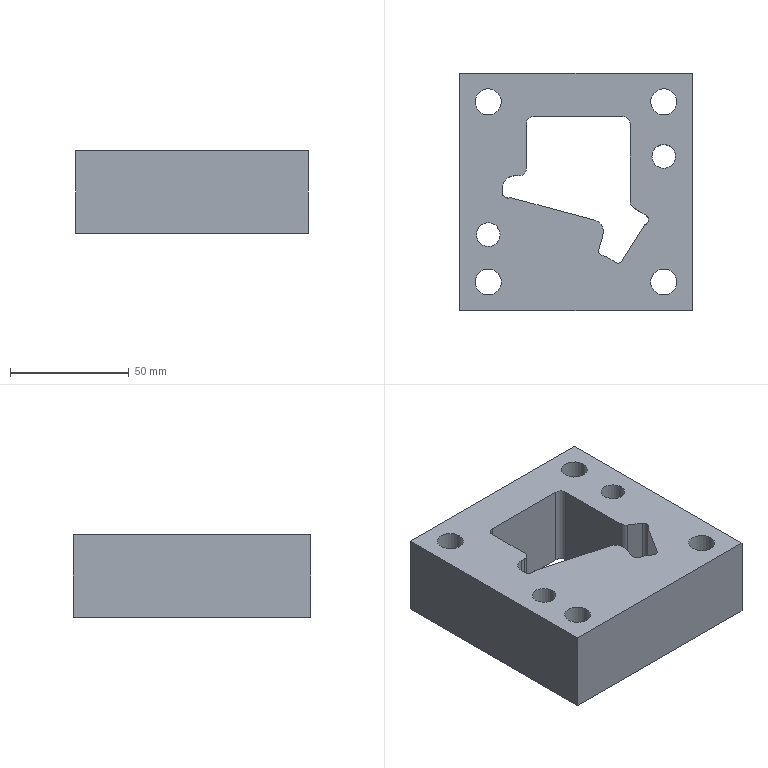Part | NX | features solid 2 | 1 solid | 52 faces | box 98 x 100 x 35 mm | volume 240089 mm3 | cylinder 27 | plane 24 | spline 1 | commonest cylinder face diameters 4 x8 11 x6 10 x5 6 x4 17 x4
STEP:
#1=CARTESIAN_POINT('',(488.719,1.701,78.));
#2=VERTEX_POINT('',#1);
#3=CARTESIAN_POINT('',(483.719,1.701,78.));
#4=DIRECTION('',(0.,0.,-1.));
#5=DIRECTION('',(1.,0.,0.));
#6=AXIS2_PLACEMENT_3D('',#3,#4,#5);
#7=CIRCLE('',#6,5.);
#8=EDGE_CURVE('',#2,#2,#7,.T.);
#9=ORIENTED_EDGE('',*,*,#8,.T.);
#10=EDGE_LOOP('',(#9));
#11=FACE_BOUND('',#10,.T.);
#12=CARTESIAN_POINT('',(414.719,-31.299,78.));
#13=VERTEX_POINT('',#12);
#14=CARTESIAN_POINT('',(409.719,-31.299,78.));
#15=DIRECTION('',(0.,0.,-1.));
#16=DIRECTION('',(1.,0.,0.));
#17=AXIS2_PLACEMENT_3D('',#14,#15,#16);
#18=CIRCLE('',#17,5.);
#19=EDGE_CURVE('',#13,#13,#18,.T.);
#20=ORIENTED_EDGE('',*,*,#19,.T.);
#21=EDGE_LOOP('',(#20));
#22=FACE_BOUND('',#21,.T.);
#23=CARTESIAN_POINT('',(415.219,-51.299,78.));
#24=VERTEX_POINT('',#23);
#25=CARTESIAN_POINT('',(409.719,-51.299,78.));
#26=DIRECTION('',(0.,0.,1.));
#27=DIRECTION('',(1.,0.,0.));
#28=AXIS2_PLACEMENT_3D('',#25,#26,#27);
#29=CIRCLE('',#28,5.5);
#30=EDGE_CURVE('',#24,#24,#29,.T.);
#31=ORIENTED_EDGE('',*,*,#30,.F.);
#32=EDGE_LOOP('',(#31));
#33=FACE_BOUND('',#32,.T.);
#34=CARTESIAN_POINT('',(478.219,-51.299,78.));
#35=VERTEX_POINT('',#34);
#36=CARTESIAN_POINT('',(483.719,-51.299,78.));
#37=DIRECTION('',(0.,0.,-1.));
#38=DIRECTION('',(-1.,0.,0.));
#39=AXIS2_PLACEMENT_3D('',#36,#37,#38);
#40=CIRCLE('',#39,5.5);
#41=EDGE_CURVE('',#35,#35,#40,.F.);
#42=ORIENTED_EDGE('',*,*,#41,.F.);
#43=EDGE_LOOP('',(#42));
#44=FACE_BOUND('',#43,.T.);
#45=CARTESIAN_POINT('',(478.219,24.701,78.));
#46=VERTEX_POINT('',#45);
#47=CARTESIAN_POINT('',(483.719,24.701,78.));
#48=DIRECTION('',(0.,0.,1.));
#49=DIRECTION('',(-1.,0.,0.));
#50=AXIS2_PLACEMENT_3D('',#47,#48,#49);
#51=CIRCLE('',#50,5.5);
#52=EDGE_CURVE('',#46,#46,#51,.T.);
#53=ORIENTED_EDGE('',*,*,#52,.F.);
#54=EDGE_LOOP('',(#53));
#55=FACE_BOUND('',#54,.T.);
#56=CARTESIAN_POINT('',(415.219,24.701,78.));
#57=VERTEX_POINT('',#56);
#58=CARTESIAN_POINT('',(409.719,24.701,78.));
#59=DIRECTION('',(0.,0.,-1.));
#60=DIRECTION('',(1.,0.,0.));
#61=AXIS2_PLACEMENT_3D('',#58,#59,#60);
#62=CIRCLE('',#61,5.5);
#63=EDGE_CURVE('',#57,#57,#62,.T.);
#64=ORIENTED_EDGE('',*,*,#63,.T.);
#65=EDGE_LOOP('',(#64));
#66=FACE_BOUND('',#65,.T.);
#67=CARTESIAN_POINT('',(495.719,36.701,78.));
#68=VERTEX_POINT('',#67);
#69=CARTESIAN_POINT('',(397.719,36.701,78.));
#70=VERTEX_POINT('',#69);
#71=CARTESIAN_POINT('',(446.479,36.701,78.));
#72=DIRECTION('',(1.,0.,0.));
#73=VECTOR('',#72,1000.);
#74=LINE('',#71,#73);
#75=EDGE_CURVE('',#68,#70,#74,.F.);
#76=ORIENTED_EDGE('',*,*,#75,.T.);
#77=CARTESIAN_POINT('',(397.719,-63.299,78.));
#78=VERTEX_POINT('',#77);
#79=CARTESIAN_POINT('',(397.719,-13.399,78.));
#80=DIRECTION('',(0.,1.,0.));
#81=VECTOR('',#80,1000.);
#82=LINE('',#79,#81);
#83=EDGE_CURVE('',#70,#78,#82,.F.);
#84=ORIENTED_EDGE('',*,*,#83,.T.);
#85=CARTESIAN_POINT('',(495.719,-63.299,78.));
#86=VERTEX_POINT('',#85);
#87=CARTESIAN_POINT('',(446.479,-63.299,78.));
#88=DIRECTION('',(-1.,0.,0.));
#89=VECTOR('',#88,1000.);
#90=LINE('',#87,#89);
#91=EDGE_CURVE('',#78,#86,#90,.F.);
#92=ORIENTED_EDGE('',*,*,#91,.T.);
#93=CARTESIAN_POINT('',(495.719,-13.399,78.));
#94=DIRECTION('',(0.,-1.,0.));
#95=VECTOR('',#94,1000.);
#96=LINE('',#93,#95);
#97=EDGE_CURVE('',#86,#68,#96,.F.);
#98=ORIENTED_EDGE('',*,*,#97,.T.);
#99=EDGE_LOOP('',(#76,#84,#92,#98));
#100=FACE_BOUND('',#99,.T.);
#101=CARTESIAN_POINT('',(420.719,-6.5,78.));
#102=VERTEX_POINT('',#101);
#103=CARTESIAN_POINT('',(415.719,-11.5,78.));
#104=VERTEX_POINT('',#103);
#105=CARTESIAN_POINT('',(420.719,-11.5,78.));
#106=DIRECTION('',(0.,0.,1.));
#107=DIRECTION('',(-1.,0.,0.));
#108=AXIS2_PLACEMENT_3D('',#105,#106,#107);
#109=CIRCLE('',#108,5.);
#110=EDGE_CURVE('',#102,#104,#109,.T.);
#111=ORIENTED_EDGE('',*,*,#110,.F.);
#112=CARTESIAN_POINT('',(422.719,-6.5,78.));
#113=VERTEX_POINT('',#112);
#114=CARTESIAN_POINT('',(396.,-6.5,78.));
#115=DIRECTION('',(1.,0.,0.));
#116=VECTOR('',#115,1000.);
#117=LINE('',#114,#116);
#118=EDGE_CURVE('',#102,#113,#117,.T.);
#119=ORIENTED_EDGE('',*,*,#118,.T.);
#120=CARTESIAN_POINT('',(425.719,-3.5,78.));
#121=VERTEX_POINT('',#120);
#122=CARTESIAN_POINT('',(422.719,-3.5,78.));
#123=DIRECTION('',(0.,0.,1.));
#124=DIRECTION('',(-1.,0.,0.));
#125=AXIS2_PLACEMENT_3D('',#122,#123,#124);
#126=CIRCLE('',#125,3.);
#127=EDGE_CURVE('',#113,#121,#126,.T.);
#128=ORIENTED_EDGE('',*,*,#127,.T.);
#129=CARTESIAN_POINT('',(425.719,15.5,78.));
#130=VERTEX_POINT('',#129);
#131=CARTESIAN_POINT('',(425.719,-6.5,78.));
#132=DIRECTION('',(0.,-1.,0.));
#133=VECTOR('',#132,1000.);
#134=LINE('',#131,#133);
#135=EDGE_CURVE('',#130,#121,#134,.T.);
#136=ORIENTED_EDGE('',*,*,#135,.F.);
#137=CARTESIAN_POINT('',(428.719,18.5,78.));
#138=VERTEX_POINT('',#137);
#139=CARTESIAN_POINT('',(428.719,15.5,78.));
#140=DIRECTION('',(0.,0.,-1.));
#141=DIRECTION('',(-1.,0.,0.));
#142=AXIS2_PLACEMENT_3D('',#139,#140,#141);
#143=CIRCLE('',#142,3.);
#144=EDGE_CURVE('',#130,#138,#143,.T.);
#145=ORIENTED_EDGE('',*,*,#144,.T.);
#146=CARTESIAN_POINT('',(466.516,18.5,78.));
#147=VERTEX_POINT('',#146);
#148=CARTESIAN_POINT('',(396.,18.5,78.));
#149=DIRECTION('',(-1.,0.,0.));
#150=VECTOR('',#149,1000.);
#151=LINE('',#148,#150);
#152=EDGE_CURVE('',#138,#147,#151,.F.);
#153=ORIENTED_EDGE('',*,*,#152,.T.);
#154=CARTESIAN_POINT('',(469.516,15.5,78.));
#155=VERTEX_POINT('',#154);
#156=CARTESIAN_POINT('',(466.516,15.5,78.));
#157=DIRECTION('',(0.,0.,-1.));
#158=DIRECTION('',(-1.,0.,0.));
#159=AXIS2_PLACEMENT_3D('',#156,#157,#158);
#160=CIRCLE('',#159,3.);
#161=EDGE_CURVE('',#147,#155,#160,.T.);
#162=ORIENTED_EDGE('',*,*,#161,.T.);
#163=CARTESIAN_POINT('',(469.516,-17.34,78.));
#164=VERTEX_POINT('',#163);
#165=CARTESIAN_POINT('',(469.516,-0.000000688,78.));
#166=DIRECTION('',(0.,1.,0.));
#167=VECTOR('',#166,1000.);
#168=LINE('',#165,#167);
#169=EDGE_CURVE('',#155,#164,#168,.F.);
#170=ORIENTED_EDGE('',*,*,#169,.T.);
#171=CARTESIAN_POINT('',(470.926,-19.884,78.));
#172=VERTEX_POINT('',#171);
#173=CARTESIAN_POINT('',(472.516,-17.34,78.));
#174=DIRECTION('',(0.,0.,1.));
#175=DIRECTION('',(-1.,0.,0.));
#176=AXIS2_PLACEMENT_3D('',#173,#174,#175);
#177=CIRCLE('',#176,3.);
#178=EDGE_CURVE('',#164,#172,#177,.T.);
#179=ORIENTED_EDGE('',*,*,#178,.T.);
#180=CARTESIAN_POINT('',(476.3,-23.242,78.));
#181=VERTEX_POINT('',#180);
#182=CARTESIAN_POINT('',(446.244,-4.461,78.));
#183=DIRECTION('',(0.848,-0.5299,0.));
#184=VECTOR('',#183,1000.);
#185=LINE('',#182,#184);
#186=EDGE_CURVE('',#172,#181,#185,.T.);
#187=ORIENTED_EDGE('',*,*,#186,.T.);
#188=CARTESIAN_POINT('',(476.937,-25.998,78.));
#189=VERTEX_POINT('',#188);
#190=CARTESIAN_POINT('',(475.24,-24.938,78.));
#191=DIRECTION('',(0.,0.,1.));
#192=DIRECTION('',(-1.,0.,0.));
#193=AXIS2_PLACEMENT_3D('',#190,#191,#192);
#194=CIRCLE('',#193,2.);
#195=EDGE_CURVE('',#189,#181,#194,.T.);
#196=ORIENTED_EDGE('',*,*,#195,.F.);
#197=CARTESIAN_POINT('',(476.732,-26.325,78.));
#198=VERTEX_POINT('',#197);
#199=CARTESIAN_POINT('',(474.858,-29.324,78.));
#200=DIRECTION('',(0.5299,0.848,0.));
#201=VECTOR('',#200,1000.);
#202=LINE('',#199,#201);
#203=EDGE_CURVE('',#198,#189,#202,.T.);
#204=ORIENTED_EDGE('',*,*,#203,.F.);
#205=CARTESIAN_POINT('',(476.007,-27.014,78.));
#206=VERTEX_POINT('',#205);
#207=CARTESIAN_POINT('',(475.036,-25.266,78.));
#208=DIRECTION('',(0.,0.,1.));
#209=DIRECTION('',(-1.,0.,0.));
#210=AXIS2_PLACEMENT_3D('',#207,#208,#209);
#211=CIRCLE('',#210,2.);
#212=EDGE_CURVE('',#206,#198,#211,.T.);
#213=ORIENTED_EDGE('',*,*,#212,.F.);
#214=CARTESIAN_POINT('',(475.282,-27.703,78.));
#215=VERTEX_POINT('',#214);
#216=CARTESIAN_POINT('',(476.978,-28.763,78.));
#217=DIRECTION('',(0.,0.,1.));
#218=DIRECTION('',(-1.,0.,0.));
#219=AXIS2_PLACEMENT_3D('',#216,#217,#218);
#220=CIRCLE('',#219,2.);
#221=EDGE_CURVE('',#215,#206,#220,.F.);
#222=ORIENTED_EDGE('',*,*,#221,.F.);
#223=CARTESIAN_POINT('',(466.124,-42.358,78.));
#224=VERTEX_POINT('',#223);
#225=CARTESIAN_POINT('',(466.124,-42.358,78.));
#226=DIRECTION('',(0.5299,0.848,0.));
#227=VECTOR('',#226,1000.);
#228=LINE('',#225,#227);
#229=EDGE_CURVE('',#224,#215,#228,.T.);
#230=ORIENTED_EDGE('',*,*,#229,.F.);
#231=CARTESIAN_POINT('',(463.368,-42.995,78.));
#232=VERTEX_POINT('',#231);
#233=CARTESIAN_POINT('',(464.428,-41.299,78.));
#234=DIRECTION('',(0.,0.,1.));
#235=DIRECTION('',(-1.,0.,0.));
#236=AXIS2_PLACEMENT_3D('',#233,#234,#235);
#237=CIRCLE('',#236,2.);
#238=EDGE_CURVE('',#224,#232,#237,.F.);
#239=ORIENTED_EDGE('',*,*,#238,.T.);
#240=CARTESIAN_POINT('',(460.057,-40.926,78.));
#241=VERTEX_POINT('',#240);
#242=CARTESIAN_POINT('',(433.735,-24.478,78.));
#243=DIRECTION('',(-0.848,0.5299,0.));
#244=VECTOR('',#243,1000.);
#245=LINE('',#242,#244);
#246=EDGE_CURVE('',#232,#241,#245,.T.);
#247=ORIENTED_EDGE('',*,*,#246,.T.);
#248=CARTESIAN_POINT('',(458.771,-40.356,78.));
#249=VERTEX_POINT('',#248);
#250=CARTESIAN_POINT('',(457.407,-45.166,78.));
#251=DIRECTION('',(0.,0.,1.));
#252=DIRECTION('',(-1.,0.,0.));
#253=AXIS2_PLACEMENT_3D('',#250,#251,#252);
#254=CIRCLE('',#253,5.);
#255=EDGE_CURVE('',#241,#249,#254,.T.);
#256=ORIENTED_EDGE('',*,*,#255,.T.);
#257=CARTESIAN_POINT('',(457.674,-40.044,78.));
#258=VERTEX_POINT('',#257);
#259=CARTESIAN_POINT('',(410.762,-26.741,78.));
#260=DIRECTION('',(-0.9621,0.2728,0.));
#261=VECTOR('',#260,1000.);
#262=LINE('',#259,#261);
#263=EDGE_CURVE('',#249,#258,#262,.T.);
#264=ORIENTED_EDGE('',*,*,#263,.T.);
#265=CARTESIAN_POINT('',(456.296,-37.575,78.));
#266=VERTEX_POINT('',#265);
#267=CARTESIAN_POINT('',(458.22,-38.12,78.));
#268=DIRECTION('',(0.,0.,1.));
#269=DIRECTION('',(-1.,0.,0.));
#270=AXIS2_PLACEMENT_3D('',#267,#268,#269);
#271=CIRCLE('',#270,2.);
#272=EDGE_CURVE('',#258,#266,#271,.F.);
#273=ORIENTED_EDGE('',*,*,#272,.T.);
#274=CARTESIAN_POINT('',(458.061,-31.404,78.));
#275=VERTEX_POINT('',#274);
#276=CARTESIAN_POINT('',(458.061,-31.404,78.));
#277=CARTESIAN_POINT('',(457.469,-33.46,78.));
#278=CARTESIAN_POINT('',(456.879,-35.516,78.));
#279=CARTESIAN_POINT('',(456.296,-37.575,78.));
#280=B_SPLINE_CURVE_WITH_KNOTS('',3,(#276,#277,#278,#279),.UNSPECIFIED.,.F.,.F.,(4,4),(0.,0.006418),.UNSPECIFIED.);
#281=EDGE_CURVE('',#275,#266,#280,.T.);
#282=ORIENTED_EDGE('',*,*,#281,.F.);
#283=CARTESIAN_POINT('',(454.551,-25.189,78.));
#284=VERTEX_POINT('',#283);
#285=CARTESIAN_POINT('',(453.257,-30.018,78.));
#286=DIRECTION('',(0.,0.,1.));
#287=DIRECTION('',(-1.,0.,0.));
#288=AXIS2_PLACEMENT_3D('',#285,#286,#287);
#289=CIRCLE('',#288,5.);
#290=EDGE_CURVE('',#284,#275,#289,.F.);
#291=ORIENTED_EDGE('',*,*,#290,.F.);
#292=CARTESIAN_POINT('',(419.626,-15.831,78.));
#293=VERTEX_POINT('',#292);
#294=CARTESIAN_POINT('',(419.626,-15.831,78.));
#295=DIRECTION('',(0.9659,-0.2588,0.));
#296=VECTOR('',#295,1000.);
#297=LINE('',#294,#296);
#298=EDGE_CURVE('',#293,#284,#297,.T.);
#299=ORIENTED_EDGE('',*,*,#298,.F.);
#300=CARTESIAN_POINT('',(418.626,-15.821,78.));
#301=VERTEX_POINT('',#300);
#302=CARTESIAN_POINT('',(419.108,-17.762,78.));
#303=DIRECTION('',(0.,0.,1.));
#304=DIRECTION('',(-1.,0.,0.));
#305=AXIS2_PLACEMENT_3D('',#302,#303,#304);
#306=CIRCLE('',#305,2.);
#307=EDGE_CURVE('',#301,#293,#306,.F.);
#308=ORIENTED_EDGE('',*,*,#307,.F.);
#309=CARTESIAN_POINT('',(417.626,-15.812,78.));
#310=VERTEX_POINT('',#309);
#311=CARTESIAN_POINT('',(418.143,-13.88,78.));
#312=DIRECTION('',(0.,0.,1.));
#313=DIRECTION('',(-1.,0.,0.));
#314=AXIS2_PLACEMENT_3D('',#311,#312,#313);
#315=CIRCLE('',#314,2.);
#316=EDGE_CURVE('',#310,#301,#315,.T.);
#317=ORIENTED_EDGE('',*,*,#316,.F.);
#318=CARTESIAN_POINT('',(417.201,-15.698,78.));
#319=VERTEX_POINT('',#318);
#320=CARTESIAN_POINT('',(402.806,-11.841,78.));
#321=DIRECTION('',(0.9659,-0.2588,0.));
#322=VECTOR('',#321,1000.);
#323=LINE('',#320,#322);
#324=EDGE_CURVE('',#319,#310,#323,.T.);
#325=ORIENTED_EDGE('',*,*,#324,.F.);
#326=CARTESIAN_POINT('',(415.719,-13.767,78.));
#327=VERTEX_POINT('',#326);
#328=CARTESIAN_POINT('',(417.719,-13.767,78.));
#329=DIRECTION('',(0.,0.,1.));
#330=DIRECTION('',(-1.,0.,0.));
#331=AXIS2_PLACEMENT_3D('',#328,#329,#330);
#332=CIRCLE('',#331,2.);
#333=EDGE_CURVE('',#327,#319,#332,.T.);
#334=ORIENTED_EDGE('',*,*,#333,.F.);
#335=CARTESIAN_POINT('',(415.719,-89.912,78.));
#336=DIRECTION('',(0.,-1.,0.));
#337=VECTOR('',#336,1000.);
#338=LINE('',#335,#337);
#339=EDGE_CURVE('',#104,#327,#338,.T.);
#340=ORIENTED_EDGE('',*,*,#339,.F.);
#341=EDGE_LOOP('',(#111,#119,#128,#136,#145,#153,#162,#170,#179,#187,#196,#204,#213,#222,#230,#239,#247,#256,#264,#273,#282,#291,#299,#308,#317,#325,#334,#340));
#342=FACE_BOUND('',#341,.T.);
#343=CARTESIAN_POINT('',(287.,-0.000000688,78.));
#344=DIRECTION('',(0.,0.,-1.));
#345=DIRECTION('',(-1.,0.,0.));
#346=AXIS2_PLACEMENT_3D('',#343,#344,#345);
#347=PLANE('',#346);
#348=ADVANCED_FACE('',(#11,#22,#33,#44,#55,#66,#100,#342),#347,.F.);
#349=CARTESIAN_POINT('',(495.719,36.701,43.));
#350=VERTEX_POINT('',#349);
#351=CARTESIAN_POINT('',(495.719,-63.299,43.));
#352=VERTEX_POINT('',#351);
#353=CARTESIAN_POINT('',(495.719,-13.399,43.));
#354=DIRECTION('',(0.,-1.,0.));
#355=VECTOR('',#354,1000.);
#356=LINE('',#353,#355);
#357=EDGE_CURVE('',#350,#352,#356,.T.);
#358=ORIENTED_EDGE('',*,*,#357,.T.);
#359=CARTESIAN_POINT('',(397.719,-63.299,43.));
#360=VERTEX_POINT('',#359);
#361=CARTESIAN_POINT('',(446.479,-63.299,43.));
#362=DIRECTION('',(-1.,0.,0.));
#363=VECTOR('',#362,1000.);
#364=LINE('',#361,#363);
#365=EDGE_CURVE('',#352,#360,#364,.T.);
#366=ORIENTED_EDGE('',*,*,#365,.T.);
#367=CARTESIAN_POINT('',(397.719,36.701,43.));
#368=VERTEX_POINT('',#367);
#369=CARTESIAN_POINT('',(397.719,-13.399,43.));
#370=DIRECTION('',(0.,1.,0.));
#371=VECTOR('',#370,1000.);
#372=LINE('',#369,#371);
#373=EDGE_CURVE('',#360,#368,#372,.T.);
#374=ORIENTED_EDGE('',*,*,#373,.T.);
#375=CARTESIAN_POINT('',(446.479,36.701,43.));
#376=DIRECTION('',(1.,0.,0.));
#377=VECTOR('',#376,1000.);
#378=LINE('',#375,#377);
#379=EDGE_CURVE('',#368,#350,#378,.T.);
#380=ORIENTED_EDGE('',*,*,#379,.T.);
#381=EDGE_LOOP('',(#358,#366,#374,#380));
#382=FACE_BOUND('',#381,.T.);
#383=CARTESIAN_POINT('',(418.219,24.701,43.));
#384=VERTEX_POINT('',#383);
#385=CARTESIAN_POINT('',(409.719,24.701,43.));
#386=DIRECTION('',(0.,0.,-1.));
#387=DIRECTION('',(1.,0.,0.));
#388=AXIS2_PLACEMENT_3D('',#385,#386,#387);
#389=CIRCLE('',#388,8.5);
#390=EDGE_CURVE('',#384,#384,#389,.T.);
#391=ORIENTED_EDGE('',*,*,#390,.F.);
#392=EDGE_LOOP('',(#391));
#393=FACE_BOUND('',#392,.T.);
#394=CARTESIAN_POINT('',(475.219,24.701,43.));
#395=VERTEX_POINT('',#394);
#396=CARTESIAN_POINT('',(483.719,24.701,43.));
#397=DIRECTION('',(0.,0.,1.));
#398=DIRECTION('',(-1.,0.,0.));
#399=AXIS2_PLACEMENT_3D('',#396,#397,#398);
#400=CIRCLE('',#399,8.5);
#401=EDGE_CURVE('',#395,#395,#400,.F.);
#402=ORIENTED_EDGE('',*,*,#401,.F.);
#403=EDGE_LOOP('',(#402));
#404=FACE_BOUND('',#403,.T.);
#405=CARTESIAN_POINT('',(475.219,-51.299,43.));
#406=VERTEX_POINT('',#405);
#407=CARTESIAN_POINT('',(483.719,-51.299,43.));
#408=DIRECTION('',(0.,0.,-1.));
#409=DIRECTION('',(-1.,0.,0.));
#410=AXIS2_PLACEMENT_3D('',#407,#408,#409);
#411=CIRCLE('',#410,8.5);
#412=EDGE_CURVE('',#406,#406,#411,.T.);
#413=ORIENTED_EDGE('',*,*,#412,.F.);
#414=EDGE_LOOP('',(#413));
#415=FACE_BOUND('',#414,.T.);
#416=CARTESIAN_POINT('',(418.219,-51.299,43.));
#417=VERTEX_POINT('',#416);
#418=CARTESIAN_POINT('',(409.719,-51.299,43.));
#419=DIRECTION('',(0.,0.,1.));
#420=DIRECTION('',(1.,0.,0.));
#421=AXIS2_PLACEMENT_3D('',#418,#419,#420);
#422=CIRCLE('',#421,8.5);
#423=EDGE_CURVE('',#417,#417,#422,.F.);
#424=ORIENTED_EDGE('',*,*,#423,.F.);
#425=EDGE_LOOP('',(#424));
#426=FACE_BOUND('',#425,.T.);
#427=CARTESIAN_POINT('',(415.219,-31.299,43.));
#428=VERTEX_POINT('',#427);
#429=CARTESIAN_POINT('',(409.719,-31.299,43.));
#430=DIRECTION('',(0.,0.,-1.));
#431=DIRECTION('',(1.,0.,0.));
#432=AXIS2_PLACEMENT_3D('',#429,#430,#431);
#433=CIRCLE('',#432,5.5);
#434=EDGE_CURVE('',#428,#428,#433,.T.);
#435=ORIENTED_EDGE('',*,*,#434,.F.);
#436=EDGE_LOOP('',(#435));
#437=FACE_BOUND('',#436,.T.);
#438=CARTESIAN_POINT('',(489.219,1.701,43.));
#439=VERTEX_POINT('',#438);
#440=CARTESIAN_POINT('',(483.719,1.701,43.));
#441=DIRECTION('',(0.,0.,-1.));
#442=DIRECTION('',(1.,0.,0.));
#443=AXIS2_PLACEMENT_3D('',#440,#441,#442);
#444=CIRCLE('',#443,5.5);
#445=EDGE_CURVE('',#439,#439,#444,.T.);
#446=ORIENTED_EDGE('',*,*,#445,.F.);
#447=EDGE_LOOP('',(#446));
#448=FACE_BOUND('',#447,.T.);
#449=CARTESIAN_POINT('',(417.201,-15.698,43.));
#450=VERTEX_POINT('',#449);
#451=CARTESIAN_POINT('',(415.719,-13.767,43.));
#452=VERTEX_POINT('',#451);
#453=CARTESIAN_POINT('',(417.719,-13.767,43.));
#454=DIRECTION('',(0.,0.,1.));
#455=DIRECTION('',(-1.,0.,0.));
#456=AXIS2_PLACEMENT_3D('',#453,#454,#455);
#457=CIRCLE('',#456,2.);
#458=EDGE_CURVE('',#450,#452,#457,.F.);
#459=ORIENTED_EDGE('',*,*,#458,.F.);
#460=CARTESIAN_POINT('',(417.626,-15.812,43.));
#461=VERTEX_POINT('',#460);
#462=CARTESIAN_POINT('',(291.797,17.903,43.));
#463=DIRECTION('',(-0.9659,0.2588,0.));
#464=VECTOR('',#463,1000.);
#465=LINE('',#462,#464);
#466=EDGE_CURVE('',#461,#450,#465,.T.);
#467=ORIENTED_EDGE('',*,*,#466,.F.);
#468=CARTESIAN_POINT('',(418.626,-15.821,43.));
#469=VERTEX_POINT('',#468);
#470=CARTESIAN_POINT('',(418.143,-13.88,43.));
#471=DIRECTION('',(0.,0.,1.));
#472=DIRECTION('',(-1.,0.,0.));
#473=AXIS2_PLACEMENT_3D('',#470,#471,#472);
#474=CIRCLE('',#473,2.);
#475=EDGE_CURVE('',#469,#461,#474,.F.);
#476=ORIENTED_EDGE('',*,*,#475,.F.);
#477=CARTESIAN_POINT('',(419.626,-15.831,43.));
#478=VERTEX_POINT('',#477);
#479=CARTESIAN_POINT('',(419.108,-17.762,43.));
#480=DIRECTION('',(0.,0.,1.));
#481=DIRECTION('',(-1.,0.,0.));
#482=AXIS2_PLACEMENT_3D('',#479,#480,#481);
#483=CIRCLE('',#482,2.);
#484=EDGE_CURVE('',#478,#469,#483,.T.);
#485=ORIENTED_EDGE('',*,*,#484,.F.);
#486=CARTESIAN_POINT('',(454.551,-25.189,43.));
#487=VERTEX_POINT('',#486);
#488=CARTESIAN_POINT('',(291.927,18.386,43.));
#489=DIRECTION('',(-0.9659,0.2588,0.));
#490=VECTOR('',#489,1000.);
#491=LINE('',#488,#490);
#492=EDGE_CURVE('',#487,#478,#491,.T.);
#493=ORIENTED_EDGE('',*,*,#492,.F.);
#494=CARTESIAN_POINT('',(458.061,-31.404,43.));
#495=VERTEX_POINT('',#494);
#496=CARTESIAN_POINT('',(453.257,-30.018,43.));
#497=DIRECTION('',(0.,0.,1.));
#498=DIRECTION('',(-1.,0.,0.));
#499=AXIS2_PLACEMENT_3D('',#496,#497,#498);
#500=CIRCLE('',#499,5.);
#501=EDGE_CURVE('',#495,#487,#500,.T.);
#502=ORIENTED_EDGE('',*,*,#501,.F.);
#503=CARTESIAN_POINT('',(456.296,-37.575,43.));
#504=VERTEX_POINT('',#503);
#505=CARTESIAN_POINT('',(456.296,-37.575,43.));
#506=CARTESIAN_POINT('',(456.879,-35.516,43.));
#507=CARTESIAN_POINT('',(457.468,-33.46,43.));
#508=CARTESIAN_POINT('',(458.061,-31.404,43.));
#509=B_SPLINE_CURVE_WITH_KNOTS('',3,(#505,#506,#507,#508),.UNSPECIFIED.,.F.,.F.,(4,4),(0.,0.006418),.UNSPECIFIED.);
#510=EDGE_CURVE('',#504,#495,#509,.T.);
#511=ORIENTED_EDGE('',*,*,#510,.F.);
#512=CARTESIAN_POINT('',(457.674,-40.044,43.));
#513=VERTEX_POINT('',#512);
#514=CARTESIAN_POINT('',(458.22,-38.12,43.));
#515=DIRECTION('',(0.,0.,1.));
#516=DIRECTION('',(-1.,0.,0.));
#517=AXIS2_PLACEMENT_3D('',#514,#515,#516);
#518=CIRCLE('',#517,2.);
#519=EDGE_CURVE('',#504,#513,#518,.T.);
#520=ORIENTED_EDGE('',*,*,#519,.T.);
#521=CARTESIAN_POINT('',(458.771,-40.356,43.));
#522=VERTEX_POINT('',#521);
#523=CARTESIAN_POINT('',(289.193,7.734,43.));
#524=DIRECTION('',(0.9621,-0.2728,0.));
#525=VECTOR('',#524,1000.);
#526=LINE('',#523,#525);
#527=EDGE_CURVE('',#513,#522,#526,.T.);
#528=ORIENTED_EDGE('',*,*,#527,.T.);
#529=CARTESIAN_POINT('',(460.057,-40.926,43.));
#530=VERTEX_POINT('',#529);
#531=CARTESIAN_POINT('',(457.407,-45.166,43.));
#532=DIRECTION('',(0.,0.,1.));
#533=DIRECTION('',(-1.,0.,0.));
#534=AXIS2_PLACEMENT_3D('',#531,#532,#533);
#535=CIRCLE('',#534,5.);
#536=EDGE_CURVE('',#530,#522,#535,.T.);
#537=ORIENTED_EDGE('',*,*,#536,.F.);
#538=CARTESIAN_POINT('',(463.368,-42.995,43.));
#539=VERTEX_POINT('',#538);
#540=CARTESIAN_POINT('',(317.205,48.338,43.));
#541=DIRECTION('',(0.848,-0.5299,0.));
#542=VECTOR('',#541,1000.);
#543=LINE('',#540,#542);
#544=EDGE_CURVE('',#530,#539,#543,.T.);
#545=ORIENTED_EDGE('',*,*,#544,.T.);
#546=CARTESIAN_POINT('',(466.124,-42.358,43.));
#547=VERTEX_POINT('',#546);
#548=CARTESIAN_POINT('',(464.428,-41.299,43.));
#549=DIRECTION('',(0.,0.,1.));
#550=DIRECTION('',(-1.,0.,0.));
#551=AXIS2_PLACEMENT_3D('',#548,#549,#550);
#552=CIRCLE('',#551,2.);
#553=EDGE_CURVE('',#539,#547,#552,.T.);
#554=ORIENTED_EDGE('',*,*,#553,.T.);
#555=CARTESIAN_POINT('',(475.282,-27.703,43.));
#556=VERTEX_POINT('',#555);
#557=CARTESIAN_POINT('',(434.859,-92.392,43.));
#558=DIRECTION('',(-0.5299,-0.848,0.));
#559=VECTOR('',#558,1000.);
#560=LINE('',#557,#559);
#561=EDGE_CURVE('',#556,#547,#560,.T.);
#562=ORIENTED_EDGE('',*,*,#561,.F.);
#563=CARTESIAN_POINT('',(476.007,-27.014,43.));
#564=VERTEX_POINT('',#563);
#565=CARTESIAN_POINT('',(476.978,-28.762,43.));
#566=DIRECTION('',(0.,0.,1.));
#567=DIRECTION('',(-1.,0.,0.));
#568=AXIS2_PLACEMENT_3D('',#565,#566,#567);
#569=CIRCLE('',#568,2.);
#570=EDGE_CURVE('',#564,#556,#569,.T.);
#571=ORIENTED_EDGE('',*,*,#570,.F.);
#572=CARTESIAN_POINT('',(476.732,-26.325,43.));
#573=VERTEX_POINT('',#572);
#574=CARTESIAN_POINT('',(475.036,-25.266,43.));
#575=DIRECTION('',(0.,0.,1.));
#576=DIRECTION('',(-1.,0.,0.));
#577=AXIS2_PLACEMENT_3D('',#574,#575,#576);
#578=CIRCLE('',#577,2.);
#579=EDGE_CURVE('',#573,#564,#578,.F.);
#580=ORIENTED_EDGE('',*,*,#579,.F.);
#581=CARTESIAN_POINT('',(476.937,-25.998,43.));
#582=VERTEX_POINT('',#581);
#583=CARTESIAN_POINT('',(435.283,-92.657,43.));
#584=DIRECTION('',(-0.5299,-0.848,0.));
#585=VECTOR('',#584,1000.);
#586=LINE('',#583,#585);
#587=EDGE_CURVE('',#582,#573,#586,.T.);
#588=ORIENTED_EDGE('',*,*,#587,.F.);
#589=CARTESIAN_POINT('',(476.3,-23.242,43.));
#590=VERTEX_POINT('',#589);
#591=CARTESIAN_POINT('',(475.24,-24.938,43.));
#592=DIRECTION('',(0.,0.,1.));
#593=DIRECTION('',(-1.,0.,0.));
#594=AXIS2_PLACEMENT_3D('',#591,#592,#593);
#595=CIRCLE('',#594,2.);
#596=EDGE_CURVE('',#590,#582,#595,.F.);
#597=ORIENTED_EDGE('',*,*,#596,.F.);
#598=CARTESIAN_POINT('',(470.926,-19.884,43.));
#599=VERTEX_POINT('',#598);
#600=CARTESIAN_POINT('',(329.713,68.356,43.));
#601=DIRECTION('',(-0.848,0.5299,0.));
#602=VECTOR('',#601,1000.);
#603=LINE('',#600,#602);
#604=EDGE_CURVE('',#590,#599,#603,.T.);
#605=ORIENTED_EDGE('',*,*,#604,.T.);
#606=CARTESIAN_POINT('',(469.516,-17.339,43.));
#607=VERTEX_POINT('',#606);
#608=CARTESIAN_POINT('',(472.516,-17.339,43.));
#609=DIRECTION('',(0.,0.,1.));
#610=DIRECTION('',(-1.,0.,0.));
#611=AXIS2_PLACEMENT_3D('',#608,#609,#610);
#612=CIRCLE('',#611,3.);
#613=EDGE_CURVE('',#607,#599,#612,.T.);
#614=ORIENTED_EDGE('',*,*,#613,.F.);
#615=CARTESIAN_POINT('',(469.516,15.5,43.));
#616=VERTEX_POINT('',#615);
#617=CARTESIAN_POINT('',(469.516,-0.000000688,43.));
#618=DIRECTION('',(0.,1.,0.));
#619=VECTOR('',#618,1000.);
#620=LINE('',#617,#619);
#621=EDGE_CURVE('',#616,#607,#620,.F.);
#622=ORIENTED_EDGE('',*,*,#621,.F.);
#623=CARTESIAN_POINT('',(466.516,18.5,43.));
#624=VERTEX_POINT('',#623);
#625=CARTESIAN_POINT('',(466.516,15.5,43.));
#626=DIRECTION('',(0.,0.,-1.));
#627=DIRECTION('',(-1.,0.,0.));
#628=AXIS2_PLACEMENT_3D('',#625,#626,#627);
#629=CIRCLE('',#628,3.);
#630=EDGE_CURVE('',#616,#624,#629,.F.);
#631=ORIENTED_EDGE('',*,*,#630,.T.);
#632=CARTESIAN_POINT('',(428.719,18.5,43.));
#633=VERTEX_POINT('',#632);
#634=CARTESIAN_POINT('',(396.,18.5,43.));
#635=DIRECTION('',(-1.,0.,0.));
#636=VECTOR('',#635,1000.);
#637=LINE('',#634,#636);
#638=EDGE_CURVE('',#624,#633,#637,.T.);
#639=ORIENTED_EDGE('',*,*,#638,.T.);
#640=CARTESIAN_POINT('',(425.719,15.5,43.));
#641=VERTEX_POINT('',#640);
#642=CARTESIAN_POINT('',(428.719,15.5,43.));
#643=DIRECTION('',(0.,0.,-1.));
#644=DIRECTION('',(-1.,0.,0.));
#645=AXIS2_PLACEMENT_3D('',#642,#643,#644);
#646=CIRCLE('',#645,3.);
#647=EDGE_CURVE('',#633,#641,#646,.F.);
#648=ORIENTED_EDGE('',*,*,#647,.T.);
#649=CARTESIAN_POINT('',(425.719,-3.5,43.));
#650=VERTEX_POINT('',#649);
#651=CARTESIAN_POINT('',(425.719,-0.000000688,43.));
#652=DIRECTION('',(0.,1.,0.));
#653=VECTOR('',#652,1000.);
#654=LINE('',#651,#653);
#655=EDGE_CURVE('',#650,#641,#654,.T.);
#656=ORIENTED_EDGE('',*,*,#655,.F.);
#657=CARTESIAN_POINT('',(422.719,-6.5,43.));
#658=VERTEX_POINT('',#657);
#659=CARTESIAN_POINT('',(422.719,-3.5,43.));
#660=DIRECTION('',(0.,0.,1.));
#661=DIRECTION('',(-1.,0.,0.));
#662=AXIS2_PLACEMENT_3D('',#659,#660,#661);
#663=CIRCLE('',#662,3.);
#664=EDGE_CURVE('',#658,#650,#663,.T.);
#665=ORIENTED_EDGE('',*,*,#664,.F.);
#666=CARTESIAN_POINT('',(420.719,-6.5,43.));
#667=VERTEX_POINT('',#666);
#668=CARTESIAN_POINT('',(287.,-6.5,43.));
#669=DIRECTION('',(-1.,0.,0.));
#670=VECTOR('',#669,1000.);
#671=LINE('',#668,#670);
#672=EDGE_CURVE('',#658,#667,#671,.T.);
#673=ORIENTED_EDGE('',*,*,#672,.T.);
#674=CARTESIAN_POINT('',(415.719,-11.5,43.));
#675=VERTEX_POINT('',#674);
#676=CARTESIAN_POINT('',(420.719,-11.5,43.));
#677=DIRECTION('',(0.,0.,1.));
#678=DIRECTION('',(-1.,0.,0.));
#679=AXIS2_PLACEMENT_3D('',#676,#677,#678);
#680=CIRCLE('',#679,5.);
#681=EDGE_CURVE('',#675,#667,#680,.F.);
#682=ORIENTED_EDGE('',*,*,#681,.F.);
#683=CARTESIAN_POINT('',(415.719,-0.000000688,43.));
#684=DIRECTION('',(0.,1.,0.));
#685=VECTOR('',#684,1000.);
#686=LINE('',#683,#685);
#687=EDGE_CURVE('',#452,#675,#686,.T.);
#688=ORIENTED_EDGE('',*,*,#687,.F.);
#689=EDGE_LOOP('',(#459,#467,#476,#485,#493,#502,#511,#520,#528,#537,#545,#554,#562,#571,#580,#588,#597,#605,#614,#622,#631,#639,#648,#656,#665,#673,#682,#688));
#690=FACE_BOUND('',#689,.T.);
#691=CARTESIAN_POINT('',(287.,-0.000000688,43.));
#692=DIRECTION('',(0.,0.,-1.));
#693=DIRECTION('',(-1.,0.,0.));
#694=AXIS2_PLACEMENT_3D('',#691,#692,#693);
#695=PLANE('',#694);
#696=ADVANCED_FACE('',(#382,#393,#404,#415,#426,#437,#448,#690),#695,.T.);
#697=CARTESIAN_POINT('',(478.219,-51.299,58.));
#698=VERTEX_POINT('',#697);
#699=CARTESIAN_POINT('',(483.719,-51.299,58.));
#700=DIRECTION('',(0.,0.,-1.));
#701=DIRECTION('',(-1.,0.,0.));
#702=AXIS2_PLACEMENT_3D('',#699,#700,#701);
#703=CIRCLE('',#702,5.5);
#704=EDGE_CURVE('',#698,#698,#703,.F.);
#705=ORIENTED_EDGE('',*,*,#704,.T.);
#706=EDGE_LOOP('',(#705));
#707=FACE_BOUND('',#706,.T.);
#708=CARTESIAN_POINT('',(475.219,-51.299,58.));
#709=VERTEX_POINT('',#708);
#710=CARTESIAN_POINT('',(483.719,-51.299,58.));
#711=DIRECTION('',(0.,0.,-1.));
#712=DIRECTION('',(-1.,0.,0.));
#713=AXIS2_PLACEMENT_3D('',#710,#711,#712);
#714=CIRCLE('',#713,8.5);
#715=EDGE_CURVE('',#709,#709,#714,.F.);
#716=ORIENTED_EDGE('',*,*,#715,.F.);
#717=EDGE_LOOP('',(#716));
#718=FACE_BOUND('',#717,.T.);
#719=CARTESIAN_POINT('',(484.086,-49.433,58.));
#720=DIRECTION('',(0.,0.,1.));
#721=DIRECTION('',(-1.,0.,0.));
#722=AXIS2_PLACEMENT_3D('',#719,#720,#721);
#723=PLANE('',#722);
#724=ADVANCED_FACE('',(#707,#718),#723,.F.);
#725=ORIENTED_EDGE('',*,*,#41,.T.);
#726=EDGE_LOOP('',(#725));
#727=FACE_BOUND('',#726,.T.);
#728=ORIENTED_EDGE('',*,*,#704,.F.);
#729=EDGE_LOOP('',(#728));
#730=FACE_BOUND('',#729,.T.);
#731=CARTESIAN_POINT('',(483.719,-51.299,78.));
#732=DIRECTION('',(0.,0.,1.));
#733=DIRECTION('',(-1.,0.,0.));
#734=AXIS2_PLACEMENT_3D('',#731,#732,#733);
#735=CYLINDRICAL_SURFACE('',#734,5.5);
#736=ADVANCED_FACE('',(#727,#730),#735,.F.);
#737=ORIENTED_EDGE('',*,*,#715,.T.);
#738=EDGE_LOOP('',(#737));
#739=FACE_BOUND('',#738,.T.);
#740=ORIENTED_EDGE('',*,*,#412,.T.);
#741=EDGE_LOOP('',(#740));
#742=FACE_BOUND('',#741,.T.);
#743=CARTESIAN_POINT('',(483.719,-51.299,43.));
#744=DIRECTION('',(0.,0.,1.));
#745=DIRECTION('',(-1.,0.,0.));
#746=AXIS2_PLACEMENT_3D('',#743,#744,#745);
#747=CYLINDRICAL_SURFACE('',#746,8.5);
#748=ADVANCED_FACE('',(#739,#742),#747,.F.);
#749=CARTESIAN_POINT('',(415.219,24.701,58.));
#750=VERTEX_POINT('',#749);
#751=CARTESIAN_POINT('',(409.719,24.701,58.));
#752=DIRECTION('',(0.,0.,-1.));
#753=DIRECTION('',(1.,0.,0.));
#754=AXIS2_PLACEMENT_3D('',#751,#752,#753);
#755=CIRCLE('',#754,5.5);
#756=EDGE_CURVE('',#750,#750,#755,.F.);
#757=ORIENTED_EDGE('',*,*,#756,.T.);
#758=EDGE_LOOP('',(#757));
#759=FACE_BOUND('',#758,.T.);
#760=CARTESIAN_POINT('',(418.219,24.701,58.));
#761=VERTEX_POINT('',#760);
#762=CARTESIAN_POINT('',(409.719,24.701,58.));
#763=DIRECTION('',(0.,0.,-1.));
#764=DIRECTION('',(1.,0.,0.));
#765=AXIS2_PLACEMENT_3D('',#762,#763,#764);
#766=CIRCLE('',#765,8.5);
#767=EDGE_CURVE('',#761,#761,#766,.F.);
#768=ORIENTED_EDGE('',*,*,#767,.F.);
#769=EDGE_LOOP('',(#768));
#770=FACE_BOUND('',#769,.T.);
#771=CARTESIAN_POINT('',(409.351,22.835,58.));
#772=DIRECTION('',(0.,0.,1.));
#773=DIRECTION('',(1.,0.,0.));
#774=AXIS2_PLACEMENT_3D('',#771,#772,#773);
#775=PLANE('',#774);
#776=ADVANCED_FACE('',(#759,#770),#775,.F.);
#777=CARTESIAN_POINT('',(478.219,24.701,58.));
#778=VERTEX_POINT('',#777);
#779=CARTESIAN_POINT('',(483.719,24.701,58.));
#780=DIRECTION('',(0.,0.,1.));
#781=DIRECTION('',(-1.,0.,0.));
#782=AXIS2_PLACEMENT_3D('',#779,#780,#781);
#783=CIRCLE('',#782,5.5);
#784=EDGE_CURVE('',#778,#778,#783,.T.);
#785=ORIENTED_EDGE('',*,*,#784,.T.);
#786=EDGE_LOOP('',(#785));
#787=FACE_BOUND('',#786,.T.);
#788=CARTESIAN_POINT('',(475.219,24.701,58.));
#789=VERTEX_POINT('',#788);
#790=CARTESIAN_POINT('',(483.719,24.701,58.));
#791=DIRECTION('',(0.,0.,1.));
#792=DIRECTION('',(-1.,0.,0.));
#793=AXIS2_PLACEMENT_3D('',#790,#791,#792);
#794=CIRCLE('',#793,8.5);
#795=EDGE_CURVE('',#789,#789,#794,.T.);
#796=ORIENTED_EDGE('',*,*,#795,.F.);
#797=EDGE_LOOP('',(#796));
#798=FACE_BOUND('',#797,.T.);
#799=CARTESIAN_POINT('',(484.086,22.835,58.));
#800=DIRECTION('',(0.,0.,1.));
#801=DIRECTION('',(-1.,0.,0.));
#802=AXIS2_PLACEMENT_3D('',#799,#800,#801);
#803=PLANE('',#802);
#804=ADVANCED_FACE('',(#787,#798),#803,.F.);
#805=CARTESIAN_POINT('',(397.719,36.701,-28.));
#806=DIRECTION('',(0.,0.,1.));
#807=VECTOR('',#806,1000.);
#808=LINE('',#805,#807);
#809=EDGE_CURVE('',#368,#70,#808,.T.);
#810=ORIENTED_EDGE('',*,*,#809,.F.);
#811=ORIENTED_EDGE('',*,*,#373,.F.);
#812=CARTESIAN_POINT('',(397.719,-63.299,-28.));
#813=DIRECTION('',(0.,0.,1.));
#814=VECTOR('',#813,1000.);
#815=LINE('',#812,#814);
#816=EDGE_CURVE('',#360,#78,#815,.T.);
#817=ORIENTED_EDGE('',*,*,#816,.T.);
#818=ORIENTED_EDGE('',*,*,#83,.F.);
#819=EDGE_LOOP('',(#810,#811,#817,#818));
#820=FACE_BOUND('',#819,.T.);
#821=CARTESIAN_POINT('',(397.719,-13.399,-28.));
#822=DIRECTION('',(-1.,0.,0.));
#823=DIRECTION('',(0.,0.,1.));
#824=AXIS2_PLACEMENT_3D('',#821,#822,#823);
#825=PLANE('',#824);
#826=ADVANCED_FACE('',(#820),#825,.T.);
#827=ORIENTED_EDGE('',*,*,#816,.F.);
#828=ORIENTED_EDGE('',*,*,#365,.F.);
#829=CARTESIAN_POINT('',(495.719,-63.299,-28.));
#830=DIRECTION('',(0.,0.,1.));
#831=VECTOR('',#830,1000.);
#832=LINE('',#829,#831);
#833=EDGE_CURVE('',#352,#86,#832,.T.);
#834=ORIENTED_EDGE('',*,*,#833,.T.);
#835=ORIENTED_EDGE('',*,*,#91,.F.);
#836=EDGE_LOOP('',(#827,#828,#834,#835));
#837=FACE_BOUND('',#836,.T.);
#838=CARTESIAN_POINT('',(446.479,-63.299,-28.));
#839=DIRECTION('',(0.,-1.,0.));
#840=DIRECTION('',(0.,0.,1.));
#841=AXIS2_PLACEMENT_3D('',#838,#839,#840);
#842=PLANE('',#841);
#843=ADVANCED_FACE('',(#837),#842,.T.);
#844=ORIENTED_EDGE('',*,*,#357,.F.);
#845=CARTESIAN_POINT('',(495.719,36.701,-28.));
#846=DIRECTION('',(0.,0.,1.));
#847=VECTOR('',#846,1000.);
#848=LINE('',#845,#847);
#849=EDGE_CURVE('',#350,#68,#848,.T.);
#850=ORIENTED_EDGE('',*,*,#849,.T.);
#851=ORIENTED_EDGE('',*,*,#97,.F.);
#852=ORIENTED_EDGE('',*,*,#833,.F.);
#853=EDGE_LOOP('',(#844,#850,#851,#852));
#854=FACE_BOUND('',#853,.T.);
#855=CARTESIAN_POINT('',(495.719,-13.399,-28.));
#856=DIRECTION('',(1.,0.,0.));
#857=DIRECTION('',(0.,0.,-1.));
#858=AXIS2_PLACEMENT_3D('',#855,#856,#857);
#859=PLANE('',#858);
#860=ADVANCED_FACE('',(#854),#859,.T.);
#861=ORIENTED_EDGE('',*,*,#849,.F.);
#862=ORIENTED_EDGE('',*,*,#379,.F.);
#863=ORIENTED_EDGE('',*,*,#809,.T.);
#864=ORIENTED_EDGE('',*,*,#75,.F.);
#865=EDGE_LOOP('',(#861,#862,#863,#864));
#866=FACE_BOUND('',#865,.T.);
#867=CARTESIAN_POINT('',(446.479,36.701,-28.));
#868=DIRECTION('',(0.,1.,0.));
#869=DIRECTION('',(0.,0.,-1.));
#870=AXIS2_PLACEMENT_3D('',#867,#868,#869);
#871=PLANE('',#870);
#872=ADVANCED_FACE('',(#866),#871,.T.);
#873=ORIENTED_EDGE('',*,*,#63,.F.);
#874=EDGE_LOOP('',(#873));
#875=FACE_BOUND('',#874,.T.);
#876=ORIENTED_EDGE('',*,*,#756,.F.);
#877=EDGE_LOOP('',(#876));
#878=FACE_BOUND('',#877,.T.);
#879=CARTESIAN_POINT('',(409.719,24.701,78.));
#880=DIRECTION('',(0.,0.,1.));
#881=DIRECTION('',(1.,0.,0.));
#882=AXIS2_PLACEMENT_3D('',#879,#880,#881);
#883=CYLINDRICAL_SURFACE('',#882,5.5);
#884=ADVANCED_FACE('',(#875,#878),#883,.F.);
#885=ORIENTED_EDGE('',*,*,#52,.T.);
#886=EDGE_LOOP('',(#885));
#887=FACE_BOUND('',#886,.T.);
#888=ORIENTED_EDGE('',*,*,#784,.F.);
#889=EDGE_LOOP('',(#888));
#890=FACE_BOUND('',#889,.T.);
#891=CARTESIAN_POINT('',(483.719,24.701,78.));
#892=DIRECTION('',(0.,0.,1.));
#893=DIRECTION('',(-1.,0.,0.));
#894=AXIS2_PLACEMENT_3D('',#891,#892,#893);
#895=CYLINDRICAL_SURFACE('',#894,5.5);
#896=ADVANCED_FACE('',(#887,#890),#895,.F.);
#897=ORIENTED_EDGE('',*,*,#767,.T.);
#898=EDGE_LOOP('',(#897));
#899=FACE_BOUND('',#898,.T.);
#900=ORIENTED_EDGE('',*,*,#390,.T.);
#901=EDGE_LOOP('',(#900));
#902=FACE_BOUND('',#901,.T.);
#903=CARTESIAN_POINT('',(409.719,24.701,43.));
#904=DIRECTION('',(0.,0.,1.));
#905=DIRECTION('',(1.,0.,0.));
#906=AXIS2_PLACEMENT_3D('',#903,#904,#905);
#907=CYLINDRICAL_SURFACE('',#906,8.5);
#908=ADVANCED_FACE('',(#899,#902),#907,.F.);
#909=ORIENTED_EDGE('',*,*,#795,.T.);
#910=EDGE_LOOP('',(#909));
#911=FACE_BOUND('',#910,.T.);
#912=ORIENTED_EDGE('',*,*,#401,.T.);
#913=EDGE_LOOP('',(#912));
#914=FACE_BOUND('',#913,.T.);
#915=CARTESIAN_POINT('',(483.719,24.701,43.));
#916=DIRECTION('',(0.,0.,1.));
#917=DIRECTION('',(-1.,0.,0.));
#918=AXIS2_PLACEMENT_3D('',#915,#916,#917);
#919=CYLINDRICAL_SURFACE('',#918,8.5);
#920=ADVANCED_FACE('',(#911,#914),#919,.F.);
#921=CARTESIAN_POINT('',(415.219,-51.299,58.));
#922=VERTEX_POINT('',#921);
#923=CARTESIAN_POINT('',(409.719,-51.299,58.));
#924=DIRECTION('',(0.,0.,1.));
#925=DIRECTION('',(1.,0.,0.));
#926=AXIS2_PLACEMENT_3D('',#923,#924,#925);
#927=CIRCLE('',#926,5.5);
#928=EDGE_CURVE('',#922,#922,#927,.T.);
#929=ORIENTED_EDGE('',*,*,#928,.T.);
#930=EDGE_LOOP('',(#929));
#931=FACE_BOUND('',#930,.T.);
#932=CARTESIAN_POINT('',(418.219,-51.299,58.));
#933=VERTEX_POINT('',#932);
#934=CARTESIAN_POINT('',(409.719,-51.299,58.));
#935=DIRECTION('',(0.,0.,1.));
#936=DIRECTION('',(1.,0.,0.));
#937=AXIS2_PLACEMENT_3D('',#934,#935,#936);
#938=CIRCLE('',#937,8.5);
#939=EDGE_CURVE('',#933,#933,#938,.T.);
#940=ORIENTED_EDGE('',*,*,#939,.F.);
#941=EDGE_LOOP('',(#940));
#942=FACE_BOUND('',#941,.T.);
#943=CARTESIAN_POINT('',(409.351,-49.433,58.));
#944=DIRECTION('',(0.,0.,1.));
#945=DIRECTION('',(1.,0.,0.));
#946=AXIS2_PLACEMENT_3D('',#943,#944,#945);
#947=PLANE('',#946);
#948=ADVANCED_FACE('',(#931,#942),#947,.F.);
#949=ORIENTED_EDGE('',*,*,#30,.T.);
#950=EDGE_LOOP('',(#949));
#951=FACE_BOUND('',#950,.T.);
#952=ORIENTED_EDGE('',*,*,#928,.F.);
#953=EDGE_LOOP('',(#952));
#954=FACE_BOUND('',#953,.T.);
#955=CARTESIAN_POINT('',(409.719,-51.299,78.));
#956=DIRECTION('',(0.,0.,1.));
#957=DIRECTION('',(1.,0.,0.));
#958=AXIS2_PLACEMENT_3D('',#955,#956,#957);
#959=CYLINDRICAL_SURFACE('',#958,5.5);
#960=ADVANCED_FACE('',(#951,#954),#959,.F.);
#961=ORIENTED_EDGE('',*,*,#939,.T.);
#962=EDGE_LOOP('',(#961));
#963=FACE_BOUND('',#962,.T.);
#964=ORIENTED_EDGE('',*,*,#423,.T.);
#965=EDGE_LOOP('',(#964));
#966=FACE_BOUND('',#965,.T.);
#967=CARTESIAN_POINT('',(409.719,-51.299,43.));
#968=DIRECTION('',(0.,0.,1.));
#969=DIRECTION('',(1.,0.,0.));
#970=AXIS2_PLACEMENT_3D('',#967,#968,#969);
#971=CYLINDRICAL_SURFACE('',#970,8.5);
#972=ADVANCED_FACE('',(#963,#966),#971,.F.);
#973=ORIENTED_EDGE('',*,*,#19,.F.);
#974=EDGE_LOOP('',(#973));
#975=FACE_BOUND('',#974,.T.);
#976=CARTESIAN_POINT('',(414.719,-31.299,58.));
#977=VERTEX_POINT('',#976);
#978=CARTESIAN_POINT('',(409.719,-31.299,58.));
#979=DIRECTION('',(0.,0.,-1.));
#980=DIRECTION('',(1.,0.,0.));
#981=AXIS2_PLACEMENT_3D('',#978,#979,#980);
#982=CIRCLE('',#981,5.);
#983=EDGE_CURVE('',#977,#977,#982,.F.);
#984=ORIENTED_EDGE('',*,*,#983,.F.);
#985=EDGE_LOOP('',(#984));
#986=FACE_BOUND('',#985,.T.);
#987=CARTESIAN_POINT('',(409.719,-31.299,78.));
#988=DIRECTION('',(0.,0.,1.));
#989=DIRECTION('',(1.,0.,0.));
#990=AXIS2_PLACEMENT_3D('',#987,#988,#989);
#991=CYLINDRICAL_SURFACE('',#990,5.);
#992=ADVANCED_FACE('',(#975,#986),#991,.F.);
#993=ORIENTED_EDGE('',*,*,#983,.T.);
#994=EDGE_LOOP('',(#993));
#995=FACE_BOUND('',#994,.T.);
#996=CARTESIAN_POINT('',(415.219,-31.299,58.));
#997=VERTEX_POINT('',#996);
#998=CARTESIAN_POINT('',(409.719,-31.299,58.));
#999=DIRECTION('',(0.,0.,-1.));
#1000=DIRECTION('',(1.,0.,0.));
#1001=AXIS2_PLACEMENT_3D('',#998,#999,#1000);
#1002=CIRCLE('',#1001,5.5);
#1003=EDGE_CURVE('',#997,#997,#1002,.F.);
#1004=ORIENTED_EDGE('',*,*,#1003,.F.);
#1005=EDGE_LOOP('',(#1004));
#1006=FACE_BOUND('',#1005,.T.);
#1007=CARTESIAN_POINT('',(410.444,-30.227,58.));
#1008=DIRECTION('',(0.,0.,1.));
#1009=DIRECTION('',(1.,0.,0.));
#1010=AXIS2_PLACEMENT_3D('',#1007,#1008,#1009);
#1011=PLANE('',#1010);
#1012=ADVANCED_FACE('',(#995,#1006),#1011,.F.);
#1013=ORIENTED_EDGE('',*,*,#1003,.T.);
#1014=EDGE_LOOP('',(#1013));
#1015=FACE_BOUND('',#1014,.T.);
#1016=ORIENTED_EDGE('',*,*,#434,.T.);
#1017=EDGE_LOOP('',(#1016));
#1018=FACE_BOUND('',#1017,.T.);
#1019=CARTESIAN_POINT('',(409.719,-31.299,43.));
#1020=DIRECTION('',(0.,0.,1.));
#1021=DIRECTION('',(1.,0.,0.));
#1022=AXIS2_PLACEMENT_3D('',#1019,#1020,#1021);
#1023=CYLINDRICAL_SURFACE('',#1022,5.5);
#1024=ADVANCED_FACE('',(#1015,#1018),#1023,.F.);
#1025=ORIENTED_EDGE('',*,*,#8,.F.);
#1026=EDGE_LOOP('',(#1025));
#1027=FACE_BOUND('',#1026,.T.);
#1028=CARTESIAN_POINT('',(488.719,1.701,58.));
#1029=VERTEX_POINT('',#1028);
#1030=CARTESIAN_POINT('',(483.719,1.701,58.));
#1031=DIRECTION('',(0.,0.,-1.));
#1032=DIRECTION('',(1.,0.,0.));
#1033=AXIS2_PLACEMENT_3D('',#1030,#1031,#1032);
#1034=CIRCLE('',#1033,5.);
#1035=EDGE_CURVE('',#1029,#1029,#1034,.F.);
#1036=ORIENTED_EDGE('',*,*,#1035,.F.);
#1037=EDGE_LOOP('',(#1036));
#1038=FACE_BOUND('',#1037,.T.);
#1039=CARTESIAN_POINT('',(483.719,1.701,78.));
#1040=DIRECTION('',(0.,0.,1.));
#1041=DIRECTION('',(1.,0.,0.));
#1042=AXIS2_PLACEMENT_3D('',#1039,#1040,#1041);
#1043=CYLINDRICAL_SURFACE('',#1042,5.);
#1044=ADVANCED_FACE('',(#1027,#1038),#1043,.F.);
#1045=ORIENTED_EDGE('',*,*,#1035,.T.);
#1046=EDGE_LOOP('',(#1045));
#1047=FACE_BOUND('',#1046,.T.);
#1048=CARTESIAN_POINT('',(489.219,1.701,58.));
#1049=VERTEX_POINT('',#1048);
#1050=CARTESIAN_POINT('',(483.719,1.701,58.));
#1051=DIRECTION('',(0.,0.,-1.));
#1052=DIRECTION('',(1.,0.,0.));
#1053=AXIS2_PLACEMENT_3D('',#1050,#1051,#1052);
#1054=CIRCLE('',#1053,5.5);
#1055=EDGE_CURVE('',#1049,#1049,#1054,.F.);
#1056=ORIENTED_EDGE('',*,*,#1055,.F.);
#1057=EDGE_LOOP('',(#1056));
#1058=FACE_BOUND('',#1057,.T.);
#1059=CARTESIAN_POINT('',(483.126,0.6285,58.));
#1060=DIRECTION('',(0.,0.,1.));
#1061=DIRECTION('',(1.,0.,0.));
#1062=AXIS2_PLACEMENT_3D('',#1059,#1060,#1061);
#1063=PLANE('',#1062);
#1064=ADVANCED_FACE('',(#1047,#1058),#1063,.F.);
#1065=ORIENTED_EDGE('',*,*,#1055,.T.);
#1066=EDGE_LOOP('',(#1065));
#1067=FACE_BOUND('',#1066,.T.);
#1068=ORIENTED_EDGE('',*,*,#445,.T.);
#1069=EDGE_LOOP('',(#1068));
#1070=FACE_BOUND('',#1069,.T.);
#1071=CARTESIAN_POINT('',(483.719,1.701,43.));
#1072=DIRECTION('',(0.,0.,1.));
#1073=DIRECTION('',(1.,0.,0.));
#1074=AXIS2_PLACEMENT_3D('',#1071,#1072,#1073);
#1075=CYLINDRICAL_SURFACE('',#1074,5.5);
#1076=ADVANCED_FACE('',(#1067,#1070),#1075,.F.);
#1077=ORIENTED_EDGE('',*,*,#604,.F.);
#1078=CARTESIAN_POINT('',(476.3,-23.242,-8.));
#1079=DIRECTION('',(0.000000369,-0.000000231,1.));
#1080=VECTOR('',#1079,1000.);
#1081=LINE('',#1078,#1080);
#1082=EDGE_CURVE('',#181,#590,#1081,.F.);
#1083=ORIENTED_EDGE('',*,*,#1082,.F.);
#1084=ORIENTED_EDGE('',*,*,#186,.F.);
#1085=CARTESIAN_POINT('',(470.926,-19.884,-8.));
#1086=DIRECTION('',(-0.000000369,0.000000231,-1.));
#1087=VECTOR('',#1086,1000.);
#1088=LINE('',#1085,#1087);
#1089=EDGE_CURVE('',#599,#172,#1088,.F.);
#1090=ORIENTED_EDGE('',*,*,#1089,.F.);
#1091=EDGE_LOOP('',(#1077,#1083,#1084,#1090));
#1092=FACE_BOUND('',#1091,.T.);
#1093=CARTESIAN_POINT('',(446.244,-4.461,-8.));
#1094=DIRECTION('',(0.5299,0.848,0.));
#1095=DIRECTION('',(0.848,-0.5299,0.));
#1096=AXIS2_PLACEMENT_3D('',#1093,#1094,#1095);
#1097=PLANE('',#1096);
#1098=ADVANCED_FACE('',(#1092),#1097,.F.);
#1099=ORIENTED_EDGE('',*,*,#169,.F.);
#1100=CARTESIAN_POINT('',(469.516,15.5,19.));
#1101=DIRECTION('',(0.000000369,-0.000000231,1.));
#1102=VECTOR('',#1101,1000.);
#1103=LINE('',#1100,#1102);
#1104=EDGE_CURVE('',#155,#616,#1103,.F.);
#1105=ORIENTED_EDGE('',*,*,#1104,.T.);
#1106=ORIENTED_EDGE('',*,*,#621,.T.);
#1107=CARTESIAN_POINT('',(469.516,-17.339,19.));
#1108=DIRECTION('',(0.000000369,-0.000000231,1.));
#1109=VECTOR('',#1108,1000.);
#1110=LINE('',#1107,#1109);
#1111=EDGE_CURVE('',#164,#607,#1110,.F.);
#1112=ORIENTED_EDGE('',*,*,#1111,.F.);
#1113=EDGE_LOOP('',(#1099,#1105,#1106,#1112));
#1114=FACE_BOUND('',#1113,.T.);
#1115=CARTESIAN_POINT('',(469.516,-119.002,19.));
#1116=DIRECTION('',(1.,0.,-0.000000369));
#1117=DIRECTION('',(-0.000000369,0.,-1.));
#1118=AXIS2_PLACEMENT_3D('',#1115,#1116,#1117);
#1119=PLANE('',#1118);
#1120=ADVANCED_FACE('',(#1114),#1119,.F.);
#1121=ORIENTED_EDGE('',*,*,#152,.F.);
#1122=CARTESIAN_POINT('',(428.719,18.5,-8.));
#1123=DIRECTION('',(0.000000369,-0.000000231,1.));
#1124=VECTOR('',#1123,1000.);
#1125=LINE('',#1122,#1124);
#1126=EDGE_CURVE('',#138,#633,#1125,.F.);
#1127=ORIENTED_EDGE('',*,*,#1126,.T.);
#1128=ORIENTED_EDGE('',*,*,#638,.F.);
#1129=CARTESIAN_POINT('',(466.516,18.5,-8.));
#1130=DIRECTION('',(-0.000000369,0.000000231,-1.));
#1131=VECTOR('',#1130,1000.);
#1132=LINE('',#1129,#1131);
#1133=EDGE_CURVE('',#624,#147,#1132,.F.);
#1134=ORIENTED_EDGE('',*,*,#1133,.T.);
#1135=EDGE_LOOP('',(#1121,#1127,#1128,#1134));
#1136=FACE_BOUND('',#1135,.T.);
#1137=CARTESIAN_POINT('',(396.,18.5,-8.));
#1138=DIRECTION('',(0.,1.,0.000000231));
#1139=DIRECTION('',(0.,0.000000231,-1.));
#1140=AXIS2_PLACEMENT_3D('',#1137,#1138,#1139);
#1141=PLANE('',#1140);
#1142=ADVANCED_FACE('',(#1136),#1141,.F.);
#1143=ORIENTED_EDGE('',*,*,#655,.T.);
#1144=CARTESIAN_POINT('',(425.719,15.5,-8.));
#1145=DIRECTION('',(0.000000369,-0.000000231,1.));
#1146=VECTOR('',#1145,1000.);
#1147=LINE('',#1144,#1146);
#1148=EDGE_CURVE('',#641,#130,#1147,.T.);
#1149=ORIENTED_EDGE('',*,*,#1148,.T.);
#1150=ORIENTED_EDGE('',*,*,#135,.T.);
#1151=CARTESIAN_POINT('',(425.719,-3.5,-8.));
#1152=DIRECTION('',(0.000000369,-0.000000231,1.));
#1153=VECTOR('',#1152,1000.);
#1154=LINE('',#1151,#1153);
#1155=EDGE_CURVE('',#650,#121,#1154,.T.);
#1156=ORIENTED_EDGE('',*,*,#1155,.F.);
#1157=EDGE_LOOP('',(#1143,#1149,#1150,#1156));
#1158=FACE_BOUND('',#1157,.T.);
#1159=CARTESIAN_POINT('',(425.719,-6.5,-8.));
#1160=DIRECTION('',(1.,0.,-0.000000369));
#1161=DIRECTION('',(0.000000369,-0.000000231,1.));
#1162=AXIS2_PLACEMENT_3D('',#1159,#1160,#1161);
#1163=PLANE('',#1162);
#1164=ADVANCED_FACE('',(#1158),#1163,.T.);
#1165=CARTESIAN_POINT('',(422.719,-6.5,-8.));
#1166=DIRECTION('',(0.000000369,-0.000000231,1.));
#1167=VECTOR('',#1166,1000.);
#1168=LINE('',#1165,#1167);
#1169=EDGE_CURVE('',#113,#658,#1168,.F.);
#1170=ORIENTED_EDGE('',*,*,#1169,.T.);
#1171=ORIENTED_EDGE('',*,*,#664,.T.);
#1172=ORIENTED_EDGE('',*,*,#1155,.T.);
#1173=ORIENTED_EDGE('',*,*,#127,.F.);
#1174=EDGE_LOOP('',(#1170,#1171,#1172,#1173));
#1175=FACE_BOUND('',#1174,.T.);
#1176=CARTESIAN_POINT('',(422.719,-3.5,-8.));
#1177=DIRECTION('',(0.000000369,-0.000000231,1.));
#1178=DIRECTION('',(1.,0.,-0.000000369));
#1179=AXIS2_PLACEMENT_3D('',#1176,#1177,#1178);
#1180=CYLINDRICAL_SURFACE('',#1179,3.);
#1181=ADVANCED_FACE('',(#1175),#1180,.T.);
#1182=ORIENTED_EDGE('',*,*,#672,.F.);
#1183=ORIENTED_EDGE('',*,*,#1169,.F.);
#1184=ORIENTED_EDGE('',*,*,#118,.F.);
#1185=CARTESIAN_POINT('',(420.719,-6.5,-8.));
#1186=DIRECTION('',(0.000000369,-0.000000231,1.));
#1187=VECTOR('',#1186,1000.);
#1188=LINE('',#1185,#1187);
#1189=EDGE_CURVE('',#102,#667,#1188,.F.);
#1190=ORIENTED_EDGE('',*,*,#1189,.T.);
#1191=EDGE_LOOP('',(#1182,#1183,#1184,#1190));
#1192=FACE_BOUND('',#1191,.T.);
#1193=CARTESIAN_POINT('',(396.,-6.5,-8.));
#1194=DIRECTION('',(0.,1.,0.000000231));
#1195=DIRECTION('',(0.,0.000000231,-1.));
#1196=AXIS2_PLACEMENT_3D('',#1193,#1194,#1195);
#1197=PLANE('',#1196);
#1198=ADVANCED_FACE('',(#1192),#1197,.F.);
#1199=ORIENTED_EDGE('',*,*,#1111,.T.);
#1200=ORIENTED_EDGE('',*,*,#613,.T.);
#1201=ORIENTED_EDGE('',*,*,#1089,.T.);
#1202=ORIENTED_EDGE('',*,*,#178,.F.);
#1203=EDGE_LOOP('',(#1199,#1200,#1201,#1202));
#1204=FACE_BOUND('',#1203,.T.);
#1205=CARTESIAN_POINT('',(472.516,-17.339,19.));
#1206=DIRECTION('',(-0.000000369,0.000000231,-1.));
#1207=DIRECTION('',(-1.,0.,0.000000369));
#1208=AXIS2_PLACEMENT_3D('',#1205,#1206,#1207);
#1209=CYLINDRICAL_SURFACE('',#1208,3.);
#1210=ADVANCED_FACE('',(#1204),#1209,.T.);
#1211=ORIENTED_EDGE('',*,*,#1082,.T.);
#1212=ORIENTED_EDGE('',*,*,#596,.T.);
#1213=CARTESIAN_POINT('',(476.936,-25.998,-8.));
#1214=DIRECTION('',(0.000000369,-0.000000231,1.));
#1215=VECTOR('',#1214,1000.);
#1216=LINE('',#1213,#1215);
#1217=EDGE_CURVE('',#189,#582,#1216,.F.);
#1218=ORIENTED_EDGE('',*,*,#1217,.F.);
#1219=ORIENTED_EDGE('',*,*,#195,.T.);
#1220=EDGE_LOOP('',(#1211,#1212,#1218,#1219));
#1221=FACE_BOUND('',#1220,.T.);
#1222=CARTESIAN_POINT('',(475.24,-24.938,-8.));
#1223=DIRECTION('',(0.000000369,-0.000000231,1.));
#1224=DIRECTION('',(1.,0.,-0.000000369));
#1225=AXIS2_PLACEMENT_3D('',#1222,#1223,#1224);
#1226=CYLINDRICAL_SURFACE('',#1225,2.);
#1227=ADVANCED_FACE('',(#1221),#1226,.F.);
#1228=ORIENTED_EDGE('',*,*,#1217,.T.);
#1229=ORIENTED_EDGE('',*,*,#587,.T.);
#1230=CARTESIAN_POINT('',(476.732,-26.325,-8.));
#1231=DIRECTION('',(0.000000369,-0.000000231,1.));
#1232=VECTOR('',#1231,1000.);
#1233=LINE('',#1230,#1232);
#1234=EDGE_CURVE('',#198,#573,#1233,.F.);
#1235=ORIENTED_EDGE('',*,*,#1234,.F.);
#1236=ORIENTED_EDGE('',*,*,#203,.T.);
#1237=EDGE_LOOP('',(#1228,#1229,#1235,#1236));
#1238=FACE_BOUND('',#1237,.T.);
#1239=CARTESIAN_POINT('',(474.858,-29.324,-8.));
#1240=DIRECTION('',(-0.848,0.5299,0.000000435));
#1241=DIRECTION('',(0.5299,0.848,0.));
#1242=AXIS2_PLACEMENT_3D('',#1239,#1240,#1241);
#1243=PLANE('',#1242);
#1244=ADVANCED_FACE('',(#1238),#1243,.T.);
#1245=ORIENTED_EDGE('',*,*,#1234,.T.);
#1246=ORIENTED_EDGE('',*,*,#579,.T.);
#1247=CARTESIAN_POINT('',(476.007,-27.014,-8.));
#1248=DIRECTION('',(0.000000369,-0.000000231,1.));
#1249=VECTOR('',#1248,1000.);
#1250=LINE('',#1247,#1249);
#1251=EDGE_CURVE('',#206,#564,#1250,.F.);
#1252=ORIENTED_EDGE('',*,*,#1251,.F.);
#1253=ORIENTED_EDGE('',*,*,#212,.T.);
#1254=EDGE_LOOP('',(#1245,#1246,#1252,#1253));
#1255=FACE_BOUND('',#1254,.T.);
#1256=CARTESIAN_POINT('',(475.036,-25.266,-8.));
#1257=DIRECTION('',(0.000000369,-0.000000231,1.));
#1258=DIRECTION('',(1.,0.,-0.000000369));
#1259=AXIS2_PLACEMENT_3D('',#1256,#1257,#1258);
#1260=CYLINDRICAL_SURFACE('',#1259,2.);
#1261=ADVANCED_FACE('',(#1255),#1260,.F.);
#1262=ORIENTED_EDGE('',*,*,#1251,.T.);
#1263=ORIENTED_EDGE('',*,*,#570,.T.);
#1264=CARTESIAN_POINT('',(475.282,-27.703,-8.));
#1265=DIRECTION('',(0.000000369,-0.000000231,1.));
#1266=VECTOR('',#1265,1000.);
#1267=LINE('',#1264,#1266);
#1268=EDGE_CURVE('',#215,#556,#1267,.F.);
#1269=ORIENTED_EDGE('',*,*,#1268,.F.);
#1270=ORIENTED_EDGE('',*,*,#221,.T.);
#1271=EDGE_LOOP('',(#1262,#1263,#1269,#1270));
#1272=FACE_BOUND('',#1271,.T.);
#1273=CARTESIAN_POINT('',(476.978,-28.762,-8.));
#1274=DIRECTION('',(0.000000369,-0.000000231,1.));
#1275=DIRECTION('',(1.,0.,-0.000000369));
#1276=AXIS2_PLACEMENT_3D('',#1273,#1274,#1275);
#1277=CYLINDRICAL_SURFACE('',#1276,2.);
#1278=ADVANCED_FACE('',(#1272),#1277,.T.);
#1279=ORIENTED_EDGE('',*,*,#1268,.T.);
#1280=ORIENTED_EDGE('',*,*,#561,.T.);
#1281=CARTESIAN_POINT('',(466.124,-42.358,82.));
#1282=DIRECTION('',(-0.000000369,0.000000231,-1.));
#1283=VECTOR('',#1282,1000.);
#1284=LINE('',#1281,#1283);
#1285=EDGE_CURVE('',#224,#547,#1284,.T.);
#1286=ORIENTED_EDGE('',*,*,#1285,.F.);
#1287=ORIENTED_EDGE('',*,*,#229,.T.);
#1288=EDGE_LOOP('',(#1279,#1280,#1286,#1287));
#1289=FACE_BOUND('',#1288,.T.);
#1290=CARTESIAN_POINT('',(466.124,-42.358,-8.));
#1291=DIRECTION('',(-0.848,0.5299,0.000000435));
#1292=DIRECTION('',(0.5299,0.848,0.));
#1293=AXIS2_PLACEMENT_3D('',#1290,#1291,#1292);
#1294=PLANE('',#1293);
#1295=ADVANCED_FACE('',(#1289),#1294,.T.);
#1296=ORIENTED_EDGE('',*,*,#553,.F.);
#1297=CARTESIAN_POINT('',(463.368,-42.995,-8.));
#1298=DIRECTION('',(-0.000000369,0.000000231,-1.));
#1299=VECTOR('',#1298,1000.);
#1300=LINE('',#1297,#1299);
#1301=EDGE_CURVE('',#539,#232,#1300,.F.);
#1302=ORIENTED_EDGE('',*,*,#1301,.T.);
#1303=ORIENTED_EDGE('',*,*,#238,.F.);
#1304=ORIENTED_EDGE('',*,*,#1285,.T.);
#1305=EDGE_LOOP('',(#1296,#1302,#1303,#1304));
#1306=FACE_BOUND('',#1305,.T.);
#1307=CARTESIAN_POINT('',(464.427,-41.299,-8.));
#1308=DIRECTION('',(0.000000369,-0.000000231,1.));
#1309=DIRECTION('',(1.,0.,-0.000000369));
#1310=AXIS2_PLACEMENT_3D('',#1307,#1308,#1309);
#1311=CYLINDRICAL_SURFACE('',#1310,2.);
#1312=ADVANCED_FACE('',(#1306),#1311,.F.);
#1313=ORIENTED_EDGE('',*,*,#544,.F.);
#1314=CARTESIAN_POINT('',(460.057,-40.926,82.));
#1315=DIRECTION('',(0.000000369,-0.000000231,1.));
#1316=VECTOR('',#1315,1000.);
#1317=LINE('',#1314,#1316);
#1318=EDGE_CURVE('',#241,#530,#1317,.F.);
#1319=ORIENTED_EDGE('',*,*,#1318,.F.);
#1320=ORIENTED_EDGE('',*,*,#246,.F.);
#1321=ORIENTED_EDGE('',*,*,#1301,.F.);
#1322=EDGE_LOOP('',(#1313,#1319,#1320,#1321));
#1323=FACE_BOUND('',#1322,.T.);
#1324=CARTESIAN_POINT('',(433.735,-24.478,-8.));
#1325=DIRECTION('',(-0.5299,-0.848,0.));
#1326=DIRECTION('',(-0.848,0.5299,0.));
#1327=AXIS2_PLACEMENT_3D('',#1324,#1325,#1326);
#1328=PLANE('',#1327);
#1329=ADVANCED_FACE('',(#1323),#1328,.F.);
#1330=ORIENTED_EDGE('',*,*,#1318,.T.);
#1331=ORIENTED_EDGE('',*,*,#536,.T.);
#1332=CARTESIAN_POINT('',(458.771,-40.356,-8.));
#1333=DIRECTION('',(0.000000369,-0.000000231,1.));
#1334=VECTOR('',#1333,1000.);
#1335=LINE('',#1332,#1334);
#1336=EDGE_CURVE('',#522,#249,#1335,.T.);
#1337=ORIENTED_EDGE('',*,*,#1336,.T.);
#1338=ORIENTED_EDGE('',*,*,#255,.F.);
#1339=EDGE_LOOP('',(#1330,#1331,#1337,#1338));
#1340=FACE_BOUND('',#1339,.T.);
#1341=CARTESIAN_POINT('',(457.407,-45.166,-8.));
#1342=DIRECTION('',(-0.000000369,0.000000231,-1.));
#1343=DIRECTION('',(-1.,0.,0.000000369));
#1344=AXIS2_PLACEMENT_3D('',#1341,#1342,#1343);
#1345=CYLINDRICAL_SURFACE('',#1344,5.);
#1346=ADVANCED_FACE('',(#1340),#1345,.T.);
#1347=ORIENTED_EDGE('',*,*,#527,.F.);
#1348=CARTESIAN_POINT('',(457.674,-40.044,82.));
#1349=DIRECTION('',(-0.000000369,0.000000231,-1.));
#1350=VECTOR('',#1349,1000.);
#1351=LINE('',#1348,#1350);
#1352=EDGE_CURVE('',#258,#513,#1351,.T.);
#1353=ORIENTED_EDGE('',*,*,#1352,.F.);
#1354=ORIENTED_EDGE('',*,*,#263,.F.);
#1355=ORIENTED_EDGE('',*,*,#1336,.F.);
#1356=EDGE_LOOP('',(#1347,#1353,#1354,#1355));
#1357=FACE_BOUND('',#1356,.T.);
#1358=CARTESIAN_POINT('',(410.762,-26.741,-8.));
#1359=DIRECTION('',(-0.2728,-0.9621,-0.000000121));
#1360=DIRECTION('',(-0.9621,0.2728,0.));
#1361=AXIS2_PLACEMENT_3D('',#1358,#1359,#1360);
#1362=PLANE('',#1361);
#1363=ADVANCED_FACE('',(#1357),#1362,.F.);
#1364=ORIENTED_EDGE('',*,*,#519,.F.);
#1365=CARTESIAN_POINT('',(456.296,-37.575,82.));
#1366=DIRECTION('',(0.000000369,-0.000000231,1.));
#1367=VECTOR('',#1366,1000.);
#1368=LINE('',#1365,#1367);
#1369=EDGE_CURVE('',#504,#266,#1368,.T.);
#1370=ORIENTED_EDGE('',*,*,#1369,.T.);
#1371=ORIENTED_EDGE('',*,*,#272,.F.);
#1372=ORIENTED_EDGE('',*,*,#1352,.T.);
#1373=EDGE_LOOP('',(#1364,#1370,#1371,#1372));
#1374=FACE_BOUND('',#1373,.T.);
#1375=CARTESIAN_POINT('',(458.22,-38.12,37.));
#1376=DIRECTION('',(0.000000369,-0.000000231,1.));
#1377=DIRECTION('',(1.,0.,-0.000000369));
#1378=AXIS2_PLACEMENT_3D('',#1375,#1376,#1377);
#1379=CYLINDRICAL_SURFACE('',#1378,2.);
#1380=ADVANCED_FACE('',(#1374),#1379,.F.);
#1381=ORIENTED_EDGE('',*,*,#1369,.F.);
#1382=ORIENTED_EDGE('',*,*,#510,.T.);
#1383=CARTESIAN_POINT('',(458.061,-31.404,-8.));
#1384=DIRECTION('',(0.000000369,-0.000000231,1.));
#1385=VECTOR('',#1384,1000.);
#1386=LINE('',#1383,#1385);
#1387=EDGE_CURVE('',#275,#495,#1386,.F.);
#1388=ORIENTED_EDGE('',*,*,#1387,.F.);
#1389=ORIENTED_EDGE('',*,*,#281,.T.);
#1390=EDGE_LOOP('',(#1381,#1382,#1388,#1389));
#1391=FACE_BOUND('',#1390,.T.);
#1392=CARTESIAN_POINT('',(458.061,-31.404,43.));
#1393=CARTESIAN_POINT('',(458.061,-31.404,78.));
#1394=CARTESIAN_POINT('',(457.468,-33.46,43.));
#1395=CARTESIAN_POINT('',(457.469,-33.46,78.));
#1396=CARTESIAN_POINT('',(456.879,-35.516,43.));
#1397=CARTESIAN_POINT('',(456.879,-35.516,78.));
#1398=CARTESIAN_POINT('',(456.296,-37.575,43.));
#1399=CARTESIAN_POINT('',(456.296,-37.575,78.));
#1400=B_SPLINE_SURFACE_WITH_KNOTS('',3,1,((#1392,#1393),(#1394,#1395),(#1396,#1397),(#1398,#1399)),.SURF_OF_LINEAR_EXTRUSION.,.F.,.F.,.F.,(4,4),(2,2),(-0.02584,0.4694),(0.,1.),.PIECEWISE_BEZIER_KNOTS.);
#1401=ADVANCED_FACE('',(#1391),#1400,.F.);
#1402=ORIENTED_EDGE('',*,*,#1387,.T.);
#1403=ORIENTED_EDGE('',*,*,#501,.T.);
#1404=CARTESIAN_POINT('',(454.551,-25.189,-8.));
#1405=DIRECTION('',(0.000000369,-0.000000231,1.));
#1406=VECTOR('',#1405,1000.);
#1407=LINE('',#1404,#1406);
#1408=EDGE_CURVE('',#284,#487,#1407,.F.);
#1409=ORIENTED_EDGE('',*,*,#1408,.F.);
#1410=ORIENTED_EDGE('',*,*,#290,.T.);
#1411=EDGE_LOOP('',(#1402,#1403,#1409,#1410));
#1412=FACE_BOUND('',#1411,.T.);
#1413=CARTESIAN_POINT('',(453.257,-30.018,-8.));
#1414=DIRECTION('',(0.000000369,-0.000000231,1.));
#1415=DIRECTION('',(1.,0.,-0.000000369));
#1416=AXIS2_PLACEMENT_3D('',#1413,#1414,#1415);
#1417=CYLINDRICAL_SURFACE('',#1416,5.);
#1418=ADVANCED_FACE('',(#1412),#1417,.T.);
#1419=ORIENTED_EDGE('',*,*,#1408,.T.);
#1420=ORIENTED_EDGE('',*,*,#492,.T.);
#1421=CARTESIAN_POINT('',(419.626,-15.83,-8.));
#1422=DIRECTION('',(0.000000369,-0.000000231,1.));
#1423=VECTOR('',#1422,1000.);
#1424=LINE('',#1421,#1423);
#1425=EDGE_CURVE('',#293,#478,#1424,.F.);
#1426=ORIENTED_EDGE('',*,*,#1425,.F.);
#1427=ORIENTED_EDGE('',*,*,#298,.T.);
#1428=EDGE_LOOP('',(#1419,#1420,#1426,#1427));
#1429=FACE_BOUND('',#1428,.T.);
#1430=CARTESIAN_POINT('',(419.626,-15.83,-8.));
#1431=DIRECTION('',(0.2588,0.9659,0.000000127));
#1432=DIRECTION('',(0.9659,-0.2588,0.));
#1433=AXIS2_PLACEMENT_3D('',#1430,#1431,#1432);
#1434=PLANE('',#1433);
#1435=ADVANCED_FACE('',(#1429),#1434,.T.);
#1436=ORIENTED_EDGE('',*,*,#1425,.T.);
#1437=ORIENTED_EDGE('',*,*,#484,.T.);
#1438=CARTESIAN_POINT('',(418.626,-15.821,-8.));
#1439=DIRECTION('',(0.000000369,-0.000000231,1.));
#1440=VECTOR('',#1439,1000.);
#1441=LINE('',#1438,#1440);
#1442=EDGE_CURVE('',#301,#469,#1441,.F.);
#1443=ORIENTED_EDGE('',*,*,#1442,.F.);
#1444=ORIENTED_EDGE('',*,*,#307,.T.);
#1445=EDGE_LOOP('',(#1436,#1437,#1443,#1444));
#1446=FACE_BOUND('',#1445,.T.);
#1447=CARTESIAN_POINT('',(419.108,-17.762,-8.));
#1448=DIRECTION('',(0.000000369,-0.000000231,1.));
#1449=DIRECTION('',(1.,0.,-0.000000369));
#1450=AXIS2_PLACEMENT_3D('',#1447,#1448,#1449);
#1451=CYLINDRICAL_SURFACE('',#1450,2.);
#1452=ADVANCED_FACE('',(#1446),#1451,.T.);
#1453=ORIENTED_EDGE('',*,*,#1442,.T.);
#1454=ORIENTED_EDGE('',*,*,#475,.T.);
#1455=CARTESIAN_POINT('',(417.626,-15.812,-8.));
#1456=DIRECTION('',(0.000000369,-0.000000231,1.));
#1457=VECTOR('',#1456,1000.);
#1458=LINE('',#1455,#1457);
#1459=EDGE_CURVE('',#310,#461,#1458,.F.);
#1460=ORIENTED_EDGE('',*,*,#1459,.F.);
#1461=ORIENTED_EDGE('',*,*,#316,.T.);
#1462=EDGE_LOOP('',(#1453,#1454,#1460,#1461));
#1463=FACE_BOUND('',#1462,.T.);
#1464=CARTESIAN_POINT('',(418.143,-13.88,-8.));
#1465=DIRECTION('',(0.000000369,-0.000000231,1.));
#1466=DIRECTION('',(1.,0.,-0.000000369));
#1467=AXIS2_PLACEMENT_3D('',#1464,#1465,#1466);
#1468=CYLINDRICAL_SURFACE('',#1467,2.);
#1469=ADVANCED_FACE('',(#1463),#1468,.F.);
#1470=ORIENTED_EDGE('',*,*,#1459,.T.);
#1471=ORIENTED_EDGE('',*,*,#466,.T.);
#1472=CARTESIAN_POINT('',(417.201,-15.698,-8.));
#1473=DIRECTION('',(0.000000369,-0.000000231,1.));
#1474=VECTOR('',#1473,1000.);
#1475=LINE('',#1472,#1474);
#1476=EDGE_CURVE('',#319,#450,#1475,.F.);
#1477=ORIENTED_EDGE('',*,*,#1476,.F.);
#1478=ORIENTED_EDGE('',*,*,#324,.T.);
#1479=EDGE_LOOP('',(#1470,#1471,#1477,#1478));
#1480=FACE_BOUND('',#1479,.T.);
#1481=CARTESIAN_POINT('',(402.806,-11.841,-8.));
#1482=DIRECTION('',(0.2588,0.9659,0.000000127));
#1483=DIRECTION('',(0.9659,-0.2588,0.));
#1484=AXIS2_PLACEMENT_3D('',#1481,#1482,#1483);
#1485=PLANE('',#1484);
#1486=ADVANCED_FACE('',(#1480),#1485,.T.);
#1487=ORIENTED_EDGE('',*,*,#1476,.T.);
#1488=ORIENTED_EDGE('',*,*,#458,.T.);
#1489=CARTESIAN_POINT('',(415.719,-13.767,-8.));
#1490=DIRECTION('',(0.000000369,-0.000000231,1.));
#1491=VECTOR('',#1490,1000.);
#1492=LINE('',#1489,#1491);
#1493=EDGE_CURVE('',#327,#452,#1492,.F.);
#1494=ORIENTED_EDGE('',*,*,#1493,.F.);
#1495=ORIENTED_EDGE('',*,*,#333,.T.);
#1496=EDGE_LOOP('',(#1487,#1488,#1494,#1495));
#1497=FACE_BOUND('',#1496,.T.);
#1498=CARTESIAN_POINT('',(417.719,-13.767,-8.));
#1499=DIRECTION('',(0.000000369,-0.000000231,1.));
#1500=DIRECTION('',(1.,0.,-0.000000369));
#1501=AXIS2_PLACEMENT_3D('',#1498,#1499,#1500);
#1502=CYLINDRICAL_SURFACE('',#1501,2.);
#1503=ADVANCED_FACE('',(#1497),#1502,.F.);
#1504=ORIENTED_EDGE('',*,*,#1493,.T.);
#1505=ORIENTED_EDGE('',*,*,#687,.T.);
#1506=CARTESIAN_POINT('',(415.719,-11.5,-8.));
#1507=DIRECTION('',(0.000000369,-0.000000231,1.));
#1508=VECTOR('',#1507,1000.);
#1509=LINE('',#1506,#1508);
#1510=EDGE_CURVE('',#104,#675,#1509,.F.);
#1511=ORIENTED_EDGE('',*,*,#1510,.F.);
#1512=ORIENTED_EDGE('',*,*,#339,.T.);
#1513=EDGE_LOOP('',(#1504,#1505,#1511,#1512));
#1514=FACE_BOUND('',#1513,.T.);
#1515=CARTESIAN_POINT('',(415.719,-89.912,-8.));
#1516=DIRECTION('',(1.,0.,-0.000000369));
#1517=DIRECTION('',(-0.000000369,0.,-1.));
#1518=AXIS2_PLACEMENT_3D('',#1515,#1516,#1517);
#1519=PLANE('',#1518);
#1520=ADVANCED_FACE('',(#1514),#1519,.T.);
#1521=ORIENTED_EDGE('',*,*,#1510,.T.);
#1522=ORIENTED_EDGE('',*,*,#681,.T.);
#1523=ORIENTED_EDGE('',*,*,#1189,.F.);
#1524=ORIENTED_EDGE('',*,*,#110,.T.);
#1525=EDGE_LOOP('',(#1521,#1522,#1523,#1524));
#1526=FACE_BOUND('',#1525,.T.);
#1527=CARTESIAN_POINT('',(420.719,-11.5,-8.));
#1528=DIRECTION('',(0.000000369,-0.000000231,1.));
#1529=DIRECTION('',(1.,0.,-0.000000369));
#1530=AXIS2_PLACEMENT_3D('',#1527,#1528,#1529);
#1531=CYLINDRICAL_SURFACE('',#1530,5.);
#1532=ADVANCED_FACE('',(#1526),#1531,.F.);
#1533=ORIENTED_EDGE('',*,*,#647,.F.);
#1534=ORIENTED_EDGE('',*,*,#1126,.F.);
#1535=ORIENTED_EDGE('',*,*,#144,.F.);
#1536=ORIENTED_EDGE('',*,*,#1148,.F.);
#1537=EDGE_LOOP('',(#1533,#1534,#1535,#1536));
#1538=FACE_BOUND('',#1537,.T.);
#1539=CARTESIAN_POINT('',(428.719,15.5,-8.));
#1540=DIRECTION('',(0.000000369,-0.000000231,1.));
#1541=DIRECTION('',(1.,0.,-0.000000369));
#1542=AXIS2_PLACEMENT_3D('',#1539,#1540,#1541);
#1543=CYLINDRICAL_SURFACE('',#1542,3.);
#1544=ADVANCED_FACE('',(#1538),#1543,.F.);
#1545=ORIENTED_EDGE('',*,*,#630,.F.);
#1546=ORIENTED_EDGE('',*,*,#1104,.F.);
#1547=ORIENTED_EDGE('',*,*,#161,.F.);
#1548=ORIENTED_EDGE('',*,*,#1133,.F.);
#1549=EDGE_LOOP('',(#1545,#1546,#1547,#1548));
#1550=FACE_BOUND('',#1549,.T.);
#1551=CARTESIAN_POINT('',(466.516,15.5,-8.));
#1552=DIRECTION('',(-0.000000369,0.000000231,-1.));
#1553=DIRECTION('',(-1.,0.,0.000000369));
#1554=AXIS2_PLACEMENT_3D('',#1551,#1552,#1553);
#1555=CYLINDRICAL_SURFACE('',#1554,3.);
#1556=ADVANCED_FACE('',(#1550),#1555,.F.);
#1557=CLOSED_SHELL('',(#348,#696,#724,#736,#748,#776,#804,#826,#843,#860,#872,#884,#896,#908,#920,#948,#960,#972,#992,#1012,#1024,#1044,#1064,#1076,#1098,#1120,#1142,#1164,#1181,#1198,#1210,#1227,#1244,#1261,#1278,#1295,#1312,#1329,#1346,#1363,#1380,#1401,#1418,#1435,#1452,#1469,#1486,#1503,#1520,#1532,#1544,#1556));
#1558=MANIFOLD_SOLID_BREP('',#1557);
#1559=(LENGTH_UNIT()NAMED_UNIT(*)SI_UNIT(.MILLI.,.METRE.));
#1560=UNCERTAINTY_MEASURE_WITH_UNIT(LENGTH_MEASURE(0.0508),#1559,'','');
#1561=(NAMED_UNIT(*)PLANE_ANGLE_UNIT()SI_UNIT($,.RADIAN.));
#1562=(NAMED_UNIT(*)SI_UNIT($,.STERADIAN.)SOLID_ANGLE_UNIT());
#1563=(GEOMETRIC_REPRESENTATION_CONTEXT(3)GLOBAL_UNCERTAINTY_ASSIGNED_CONTEXT((#1560))GLOBAL_UNIT_ASSIGNED_CONTEXT((#1559,#1561,#1562))REPRESENTATION_CONTEXT('',''));
#1564=ADVANCED_BREP_SHAPE_REPRESENTATION('',(#1558),#1563);